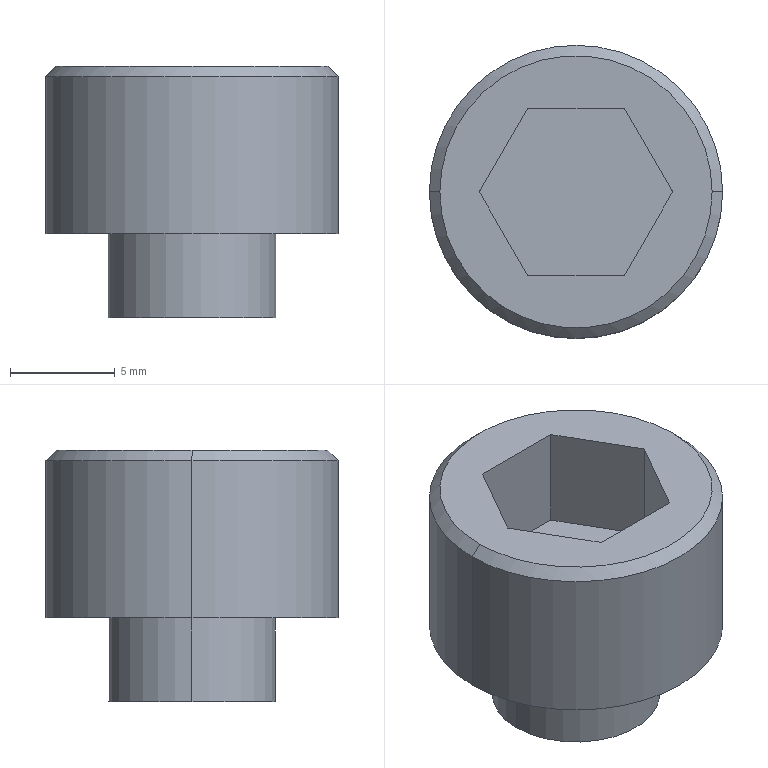Part | NX | 1 solid | 16 faces | box 14 x 14 x 12 mm | volume 1150 mm3 | plane 10 | cylinder 4 | cone 2 | commonest cylinder face diameters 8 x2 14 x2
STEP:
#1=CARTESIAN_POINT('',(6.5,0.,0.));
#2=VERTEX_POINT('',#1);
#3=CARTESIAN_POINT('',(-6.5,0.,0.));
#4=VERTEX_POINT('',#3);
#5=CARTESIAN_POINT('',(0.,0.,0.));
#6=DIRECTION('',(0.,0.,1.));
#7=DIRECTION('',(1.,0.,0.));
#8=AXIS2_PLACEMENT_3D('',#5,#6,#7);
#9=CIRCLE('',#8,6.5);
#10=EDGE_CURVE('',#2,#4,#9,.T.);
#11=ORIENTED_EDGE('',*,*,#10,.F.);
#12=CARTESIAN_POINT('',(7.,0.,-0.5));
#13=VERTEX_POINT('',#12);
#14=CARTESIAN_POINT('',(6.5,0.,0.));
#15=DIRECTION('',(-0.7071,0.,0.7071));
#16=VECTOR('',#15,1.);
#17=LINE('',#14,#16);
#18=EDGE_CURVE('',#13,#2,#17,.T.);
#19=ORIENTED_EDGE('',*,*,#18,.F.);
#20=CARTESIAN_POINT('',(-7.,0.,-0.5));
#21=VERTEX_POINT('',#20);
#22=CARTESIAN_POINT('',(0.,0.,-0.5));
#23=DIRECTION('',(0.,0.,-1.));
#24=DIRECTION('',(1.,0.,0.));
#25=AXIS2_PLACEMENT_3D('',#22,#23,#24);
#26=CIRCLE('',#25,7.);
#27=EDGE_CURVE('',#21,#13,#26,.T.);
#28=ORIENTED_EDGE('',*,*,#27,.F.);
#29=CARTESIAN_POINT('',(-6.5,0.,0.));
#30=DIRECTION('',(0.7071,0.,0.7071));
#31=VECTOR('',#30,1.);
#32=LINE('',#29,#31);
#33=EDGE_CURVE('',#21,#4,#32,.T.);
#34=ORIENTED_EDGE('',*,*,#33,.T.);
#35=EDGE_LOOP('',(#11,#19,#28,#34));
#36=FACE_OUTER_BOUND('',#35,.T.);
#37=CARTESIAN_POINT('',(0.,0.,0.));
#38=DIRECTION('',(0.,0.,-1.));
#39=DIRECTION('',(-1.,0.,0.));
#40=AXIS2_PLACEMENT_3D('',#37,#38,#39);
#41=CONICAL_SURFACE('',#40,6.5,45.);
#42=ADVANCED_FACE('',(#36),#41,.T.);
#43=CARTESIAN_POINT('',(-4.,0.,-12.));
#44=VERTEX_POINT('',#43);
#45=CARTESIAN_POINT('',(4.,0.,-12.));
#46=VERTEX_POINT('',#45);
#47=CARTESIAN_POINT('',(0.,0.,-12.));
#48=DIRECTION('',(0.,0.,-1.));
#49=DIRECTION('',(-1.,0.,0.));
#50=AXIS2_PLACEMENT_3D('',#47,#48,#49);
#51=CIRCLE('',#50,4.);
#52=EDGE_CURVE('',#44,#46,#51,.T.);
#53=ORIENTED_EDGE('',*,*,#52,.F.);
#54=CARTESIAN_POINT('',(-4.,0.,-8.));
#55=VERTEX_POINT('',#54);
#56=CARTESIAN_POINT('',(-4.,0.,-12.));
#57=DIRECTION('',(0.,0.,1.));
#58=VECTOR('',#57,1.);
#59=LINE('',#56,#58);
#60=EDGE_CURVE('',#44,#55,#59,.T.);
#61=ORIENTED_EDGE('',*,*,#60,.T.);
#62=CARTESIAN_POINT('',(4.,0.,-8.));
#63=VERTEX_POINT('',#62);
#64=CARTESIAN_POINT('',(0.,0.,-8.));
#65=DIRECTION('',(0.,0.,-1.));
#66=DIRECTION('',(1.,0.,0.));
#67=AXIS2_PLACEMENT_3D('',#64,#65,#66);
#68=CIRCLE('',#67,4.);
#69=EDGE_CURVE('',#55,#63,#68,.T.);
#70=ORIENTED_EDGE('',*,*,#69,.T.);
#71=CARTESIAN_POINT('',(4.,0.,-12.));
#72=DIRECTION('',(0.,0.,1.));
#73=VECTOR('',#72,1.);
#74=LINE('',#71,#73);
#75=EDGE_CURVE('',#46,#63,#74,.T.);
#76=ORIENTED_EDGE('',*,*,#75,.F.);
#77=EDGE_LOOP('',(#53,#61,#70,#76));
#78=FACE_OUTER_BOUND('',#77,.T.);
#79=CARTESIAN_POINT('',(0.,0.,-12.));
#80=DIRECTION('',(0.,0.,1.));
#81=DIRECTION('',(1.,0.,0.));
#82=AXIS2_PLACEMENT_3D('',#79,#80,#81);
#83=CYLINDRICAL_SURFACE('',#82,4.);
#84=ADVANCED_FACE('',(#78),#83,.T.);
#85=CARTESIAN_POINT('',(7.,0.,-8.));
#86=VERTEX_POINT('',#85);
#87=CARTESIAN_POINT('',(-7.,0.,-8.));
#88=VERTEX_POINT('',#87);
#89=CARTESIAN_POINT('',(0.,0.,-8.));
#90=DIRECTION('',(0.,0.,1.));
#91=DIRECTION('',(1.,0.,0.));
#92=AXIS2_PLACEMENT_3D('',#89,#90,#91);
#93=CIRCLE('',#92,7.);
#94=EDGE_CURVE('',#86,#88,#93,.T.);
#95=ORIENTED_EDGE('',*,*,#94,.T.);
#96=CARTESIAN_POINT('',(-7.,0.,-8.));
#97=DIRECTION('',(0.,0.,1.));
#98=VECTOR('',#97,1.);
#99=LINE('',#96,#98);
#100=EDGE_CURVE('',#88,#21,#99,.T.);
#101=ORIENTED_EDGE('',*,*,#100,.T.);
#102=ORIENTED_EDGE('',*,*,#27,.T.);
#103=CARTESIAN_POINT('',(7.,0.,-8.));
#104=DIRECTION('',(0.,0.,1.));
#105=VECTOR('',#104,1.);
#106=LINE('',#103,#105);
#107=EDGE_CURVE('',#86,#13,#106,.T.);
#108=ORIENTED_EDGE('',*,*,#107,.F.);
#109=EDGE_LOOP('',(#95,#101,#102,#108));
#110=FACE_OUTER_BOUND('',#109,.T.);
#111=CARTESIAN_POINT('',(0.,0.,-8.));
#112=DIRECTION('',(0.,0.,1.));
#113=DIRECTION('',(1.,0.,0.));
#114=AXIS2_PLACEMENT_3D('',#111,#112,#113);
#115=CYLINDRICAL_SURFACE('',#114,7.);
#116=ADVANCED_FACE('',(#110),#115,.T.);
#117=ORIENTED_EDGE('',*,*,#94,.F.);
#118=CARTESIAN_POINT('',(0.,0.,-8.));
#119=DIRECTION('',(0.,0.,1.));
#120=DIRECTION('',(1.,0.,0.));
#121=AXIS2_PLACEMENT_3D('',#118,#119,#120);
#122=CIRCLE('',#121,7.);
#123=EDGE_CURVE('',#88,#86,#122,.T.);
#124=ORIENTED_EDGE('',*,*,#123,.F.);
#125=EDGE_LOOP('',(#117,#124));
#126=FACE_BOUND('',#125,.T.);
#127=CARTESIAN_POINT('',(0.,0.,-8.));
#128=DIRECTION('',(0.,0.,-1.));
#129=DIRECTION('',(1.,0.,0.));
#130=AXIS2_PLACEMENT_3D('',#127,#128,#129);
#131=CIRCLE('',#130,4.);
#132=EDGE_CURVE('',#63,#55,#131,.T.);
#133=ORIENTED_EDGE('',*,*,#132,.F.);
#134=ORIENTED_EDGE('',*,*,#69,.F.);
#135=EDGE_LOOP('',(#133,#134));
#136=FACE_BOUND('',#135,.T.);
#137=CARTESIAN_POINT('',(0.,0.,-8.));
#138=DIRECTION('',(0.,0.,1.));
#139=DIRECTION('',(1.,0.,0.));
#140=AXIS2_PLACEMENT_3D('',#137,#138,#139);
#141=PLANE('',#140);
#142=ADVANCED_FACE('',(#126,#136),#141,.F.);
#143=ORIENTED_EDGE('',*,*,#100,.F.);
#144=ORIENTED_EDGE('',*,*,#123,.T.);
#145=ORIENTED_EDGE('',*,*,#107,.T.);
#146=CARTESIAN_POINT('',(0.,0.,-0.5));
#147=DIRECTION('',(0.,0.,-1.));
#148=DIRECTION('',(1.,0.,0.));
#149=AXIS2_PLACEMENT_3D('',#146,#147,#148);
#150=CIRCLE('',#149,7.);
#151=EDGE_CURVE('',#13,#21,#150,.T.);
#152=ORIENTED_EDGE('',*,*,#151,.T.);
#153=EDGE_LOOP('',(#143,#144,#145,#152));
#154=FACE_OUTER_BOUND('',#153,.T.);
#155=CARTESIAN_POINT('',(0.,0.,-8.));
#156=DIRECTION('',(0.,0.,1.));
#157=DIRECTION('',(1.,0.,0.));
#158=AXIS2_PLACEMENT_3D('',#155,#156,#157);
#159=CYLINDRICAL_SURFACE('',#158,7.);
#160=ADVANCED_FACE('',(#154),#159,.T.);
#161=CARTESIAN_POINT('',(2.309,-4.,0.));
#162=VERTEX_POINT('',#161);
#163=CARTESIAN_POINT('',(4.619,0.,0.));
#164=VERTEX_POINT('',#163);
#165=CARTESIAN_POINT('',(2.309,-4.,0.));
#166=DIRECTION('',(0.5,0.866,0.));
#167=VECTOR('',#166,1.);
#168=LINE('',#165,#167);
#169=EDGE_CURVE('',#162,#164,#168,.T.);
#170=ORIENTED_EDGE('',*,*,#169,.F.);
#171=CARTESIAN_POINT('',(-2.309,-4.,0.));
#172=VERTEX_POINT('',#171);
#173=CARTESIAN_POINT('',(-2.309,-4.,0.));
#174=DIRECTION('',(1.,0.,0.));
#175=VECTOR('',#174,1.);
#176=LINE('',#173,#175);
#177=EDGE_CURVE('',#172,#162,#176,.T.);
#178=ORIENTED_EDGE('',*,*,#177,.F.);
#179=CARTESIAN_POINT('',(-4.619,0.,0.));
#180=VERTEX_POINT('',#179);
#181=CARTESIAN_POINT('',(-4.619,0.,0.));
#182=DIRECTION('',(0.5,-0.866,0.));
#183=VECTOR('',#182,1.);
#184=LINE('',#181,#183);
#185=EDGE_CURVE('',#180,#172,#184,.T.);
#186=ORIENTED_EDGE('',*,*,#185,.F.);
#187=CARTESIAN_POINT('',(-2.309,4.,0.));
#188=VERTEX_POINT('',#187);
#189=CARTESIAN_POINT('',(-2.309,4.,0.));
#190=DIRECTION('',(-0.5,-0.866,0.));
#191=VECTOR('',#190,1.);
#192=LINE('',#189,#191);
#193=EDGE_CURVE('',#188,#180,#192,.T.);
#194=ORIENTED_EDGE('',*,*,#193,.F.);
#195=CARTESIAN_POINT('',(2.309,4.,0.));
#196=VERTEX_POINT('',#195);
#197=CARTESIAN_POINT('',(2.309,4.,0.));
#198=DIRECTION('',(-1.,0.,0.));
#199=VECTOR('',#198,1.);
#200=LINE('',#197,#199);
#201=EDGE_CURVE('',#196,#188,#200,.T.);
#202=ORIENTED_EDGE('',*,*,#201,.F.);
#203=CARTESIAN_POINT('',(4.619,0.,0.));
#204=DIRECTION('',(-0.5,0.866,0.));
#205=VECTOR('',#204,1.);
#206=LINE('',#203,#205);
#207=EDGE_CURVE('',#164,#196,#206,.T.);
#208=ORIENTED_EDGE('',*,*,#207,.F.);
#209=EDGE_LOOP('',(#170,#178,#186,#194,#202,#208));
#210=FACE_BOUND('',#209,.T.);
#211=CARTESIAN_POINT('',(0.,0.,0.));
#212=DIRECTION('',(0.,0.,1.));
#213=DIRECTION('',(1.,0.,0.));
#214=AXIS2_PLACEMENT_3D('',#211,#212,#213);
#215=CIRCLE('',#214,6.5);
#216=EDGE_CURVE('',#4,#2,#215,.T.);
#217=ORIENTED_EDGE('',*,*,#216,.T.);
#218=ORIENTED_EDGE('',*,*,#10,.T.);
#219=EDGE_LOOP('',(#217,#218));
#220=FACE_BOUND('',#219,.T.);
#221=CARTESIAN_POINT('',(0.,0.,0.));
#222=DIRECTION('',(0.,0.,1.));
#223=DIRECTION('',(1.,0.,0.));
#224=AXIS2_PLACEMENT_3D('',#221,#222,#223);
#225=PLANE('',#224);
#226=ADVANCED_FACE('',(#210,#220),#225,.T.);
#227=ORIENTED_EDGE('',*,*,#60,.F.);
#228=CARTESIAN_POINT('',(0.,0.,-12.));
#229=DIRECTION('',(0.,0.,-1.));
#230=DIRECTION('',(-1.,0.,0.));
#231=AXIS2_PLACEMENT_3D('',#228,#229,#230);
#232=CIRCLE('',#231,4.);
#233=EDGE_CURVE('',#46,#44,#232,.T.);
#234=ORIENTED_EDGE('',*,*,#233,.F.);
#235=ORIENTED_EDGE('',*,*,#75,.T.);
#236=ORIENTED_EDGE('',*,*,#132,.T.);
#237=EDGE_LOOP('',(#227,#234,#235,#236));
#238=FACE_OUTER_BOUND('',#237,.T.);
#239=CARTESIAN_POINT('',(0.,0.,-12.));
#240=DIRECTION('',(0.,0.,1.));
#241=DIRECTION('',(1.,0.,0.));
#242=AXIS2_PLACEMENT_3D('',#239,#240,#241);
#243=CYLINDRICAL_SURFACE('',#242,4.);
#244=ADVANCED_FACE('',(#238),#243,.T.);
#245=ORIENTED_EDGE('',*,*,#233,.T.);
#246=ORIENTED_EDGE('',*,*,#52,.T.);
#247=EDGE_LOOP('',(#245,#246));
#248=FACE_OUTER_BOUND('',#247,.T.);
#249=CARTESIAN_POINT('',(0.,0.,-12.));
#250=DIRECTION('',(0.,0.,-1.));
#251=DIRECTION('',(-1.,0.,0.));
#252=AXIS2_PLACEMENT_3D('',#249,#250,#251);
#253=PLANE('',#252);
#254=ADVANCED_FACE('',(#248),#253,.T.);
#255=ORIENTED_EDGE('',*,*,#18,.T.);
#256=ORIENTED_EDGE('',*,*,#216,.F.);
#257=ORIENTED_EDGE('',*,*,#33,.F.);
#258=ORIENTED_EDGE('',*,*,#151,.F.);
#259=EDGE_LOOP('',(#255,#256,#257,#258));
#260=FACE_OUTER_BOUND('',#259,.T.);
#261=CARTESIAN_POINT('',(0.,0.,0.));
#262=DIRECTION('',(0.,0.,-1.));
#263=DIRECTION('',(-1.,0.,0.));
#264=AXIS2_PLACEMENT_3D('',#261,#262,#263);
#265=CONICAL_SURFACE('',#264,6.5,45.);
#266=ADVANCED_FACE('',(#260),#265,.T.);
#267=ORIENTED_EDGE('',*,*,#169,.T.);
#268=CARTESIAN_POINT('',(4.619,0.,-5.));
#269=VERTEX_POINT('',#268);
#270=CARTESIAN_POINT('',(4.619,0.,-5.));
#271=DIRECTION('',(0.,0.,1.));
#272=VECTOR('',#271,1.);
#273=LINE('',#270,#272);
#274=EDGE_CURVE('',#269,#164,#273,.T.);
#275=ORIENTED_EDGE('',*,*,#274,.F.);
#276=CARTESIAN_POINT('',(2.309,-4.,-5.));
#277=VERTEX_POINT('',#276);
#278=CARTESIAN_POINT('',(2.309,-4.,-5.));
#279=DIRECTION('',(0.5,0.866,0.));
#280=VECTOR('',#279,1.);
#281=LINE('',#278,#280);
#282=EDGE_CURVE('',#277,#269,#281,.T.);
#283=ORIENTED_EDGE('',*,*,#282,.F.);
#284=CARTESIAN_POINT('',(2.309,-4.,-5.));
#285=DIRECTION('',(0.,0.,1.));
#286=VECTOR('',#285,1.);
#287=LINE('',#284,#286);
#288=EDGE_CURVE('',#277,#162,#287,.T.);
#289=ORIENTED_EDGE('',*,*,#288,.T.);
#290=EDGE_LOOP('',(#267,#275,#283,#289));
#291=FACE_OUTER_BOUND('',#290,.T.);
#292=CARTESIAN_POINT('',(2.309,-4.,-5.));
#293=DIRECTION('',(0.866,-0.5,0.));
#294=DIRECTION('',(0.5,0.866,0.));
#295=AXIS2_PLACEMENT_3D('',#292,#293,#294);
#296=PLANE('',#295);
#297=ADVANCED_FACE('',(#291),#296,.F.);
#298=ORIENTED_EDGE('',*,*,#177,.T.);
#299=ORIENTED_EDGE('',*,*,#288,.F.);
#300=CARTESIAN_POINT('',(-2.309,-4.,-5.));
#301=VERTEX_POINT('',#300);
#302=CARTESIAN_POINT('',(-2.309,-4.,-5.));
#303=DIRECTION('',(1.,0.,0.));
#304=VECTOR('',#303,1.);
#305=LINE('',#302,#304);
#306=EDGE_CURVE('',#301,#277,#305,.T.);
#307=ORIENTED_EDGE('',*,*,#306,.F.);
#308=CARTESIAN_POINT('',(-2.309,-4.,-5.));
#309=DIRECTION('',(0.,0.,1.));
#310=VECTOR('',#309,1.);
#311=LINE('',#308,#310);
#312=EDGE_CURVE('',#301,#172,#311,.T.);
#313=ORIENTED_EDGE('',*,*,#312,.T.);
#314=EDGE_LOOP('',(#298,#299,#307,#313));
#315=FACE_OUTER_BOUND('',#314,.T.);
#316=CARTESIAN_POINT('',(-2.309,-4.,-5.));
#317=DIRECTION('',(0.,-1.,0.));
#318=DIRECTION('',(0.,0.,-1.));
#319=AXIS2_PLACEMENT_3D('',#316,#317,#318);
#320=PLANE('',#319);
#321=ADVANCED_FACE('',(#315),#320,.F.);
#322=ORIENTED_EDGE('',*,*,#185,.T.);
#323=ORIENTED_EDGE('',*,*,#312,.F.);
#324=CARTESIAN_POINT('',(-4.619,0.,-5.));
#325=VERTEX_POINT('',#324);
#326=CARTESIAN_POINT('',(-4.619,0.,-5.));
#327=DIRECTION('',(0.5,-0.866,0.));
#328=VECTOR('',#327,1.);
#329=LINE('',#326,#328);
#330=EDGE_CURVE('',#325,#301,#329,.T.);
#331=ORIENTED_EDGE('',*,*,#330,.F.);
#332=CARTESIAN_POINT('',(-4.619,0.,-5.));
#333=DIRECTION('',(0.,0.,1.));
#334=VECTOR('',#333,1.);
#335=LINE('',#332,#334);
#336=EDGE_CURVE('',#325,#180,#335,.T.);
#337=ORIENTED_EDGE('',*,*,#336,.T.);
#338=EDGE_LOOP('',(#322,#323,#331,#337));
#339=FACE_OUTER_BOUND('',#338,.T.);
#340=CARTESIAN_POINT('',(-4.619,0.,-5.));
#341=DIRECTION('',(-0.866,-0.5,0.));
#342=DIRECTION('',(0.5,-0.866,0.));
#343=AXIS2_PLACEMENT_3D('',#340,#341,#342);
#344=PLANE('',#343);
#345=ADVANCED_FACE('',(#339),#344,.F.);
#346=ORIENTED_EDGE('',*,*,#193,.T.);
#347=ORIENTED_EDGE('',*,*,#336,.F.);
#348=CARTESIAN_POINT('',(-2.309,4.,-5.));
#349=VERTEX_POINT('',#348);
#350=CARTESIAN_POINT('',(-2.309,4.,-5.));
#351=DIRECTION('',(-0.5,-0.866,0.));
#352=VECTOR('',#351,1.);
#353=LINE('',#350,#352);
#354=EDGE_CURVE('',#349,#325,#353,.T.);
#355=ORIENTED_EDGE('',*,*,#354,.F.);
#356=CARTESIAN_POINT('',(-2.309,4.,-5.));
#357=DIRECTION('',(0.,0.,1.));
#358=VECTOR('',#357,1.);
#359=LINE('',#356,#358);
#360=EDGE_CURVE('',#349,#188,#359,.T.);
#361=ORIENTED_EDGE('',*,*,#360,.T.);
#362=EDGE_LOOP('',(#346,#347,#355,#361));
#363=FACE_OUTER_BOUND('',#362,.T.);
#364=CARTESIAN_POINT('',(-2.309,4.,-5.));
#365=DIRECTION('',(-0.866,0.5,0.));
#366=DIRECTION('',(-0.5,-0.866,0.));
#367=AXIS2_PLACEMENT_3D('',#364,#365,#366);
#368=PLANE('',#367);
#369=ADVANCED_FACE('',(#363),#368,.F.);
#370=ORIENTED_EDGE('',*,*,#201,.T.);
#371=ORIENTED_EDGE('',*,*,#360,.F.);
#372=CARTESIAN_POINT('',(2.309,4.,-5.));
#373=VERTEX_POINT('',#372);
#374=CARTESIAN_POINT('',(2.309,4.,-5.));
#375=DIRECTION('',(-1.,0.,0.));
#376=VECTOR('',#375,1.);
#377=LINE('',#374,#376);
#378=EDGE_CURVE('',#373,#349,#377,.T.);
#379=ORIENTED_EDGE('',*,*,#378,.F.);
#380=CARTESIAN_POINT('',(2.309,4.,-5.));
#381=DIRECTION('',(0.,0.,1.));
#382=VECTOR('',#381,1.);
#383=LINE('',#380,#382);
#384=EDGE_CURVE('',#373,#196,#383,.T.);
#385=ORIENTED_EDGE('',*,*,#384,.T.);
#386=EDGE_LOOP('',(#370,#371,#379,#385));
#387=FACE_OUTER_BOUND('',#386,.T.);
#388=CARTESIAN_POINT('',(2.309,4.,-5.));
#389=DIRECTION('',(0.,1.,0.));
#390=DIRECTION('',(-1.,0.,0.));
#391=AXIS2_PLACEMENT_3D('',#388,#389,#390);
#392=PLANE('',#391);
#393=ADVANCED_FACE('',(#387),#392,.F.);
#394=ORIENTED_EDGE('',*,*,#207,.T.);
#395=ORIENTED_EDGE('',*,*,#384,.F.);
#396=CARTESIAN_POINT('',(4.619,0.,-5.));
#397=DIRECTION('',(-0.5,0.866,0.));
#398=VECTOR('',#397,1.);
#399=LINE('',#396,#398);
#400=EDGE_CURVE('',#269,#373,#399,.T.);
#401=ORIENTED_EDGE('',*,*,#400,.F.);
#402=ORIENTED_EDGE('',*,*,#274,.T.);
#403=EDGE_LOOP('',(#394,#395,#401,#402));
#404=FACE_OUTER_BOUND('',#403,.T.);
#405=CARTESIAN_POINT('',(4.619,0.,-5.));
#406=DIRECTION('',(0.866,0.5,0.));
#407=DIRECTION('',(-0.5,0.866,0.));
#408=AXIS2_PLACEMENT_3D('',#405,#406,#407);
#409=PLANE('',#408);
#410=ADVANCED_FACE('',(#404),#409,.F.);
#411=ORIENTED_EDGE('',*,*,#282,.T.);
#412=ORIENTED_EDGE('',*,*,#400,.T.);
#413=ORIENTED_EDGE('',*,*,#378,.T.);
#414=ORIENTED_EDGE('',*,*,#354,.T.);
#415=ORIENTED_EDGE('',*,*,#330,.T.);
#416=ORIENTED_EDGE('',*,*,#306,.T.);
#417=EDGE_LOOP('',(#411,#412,#413,#414,#415,#416));
#418=FACE_OUTER_BOUND('',#417,.T.);
#419=CARTESIAN_POINT('',(0.,0.,-5.));
#420=DIRECTION('',(0.,0.,1.));
#421=DIRECTION('',(1.,0.,0.));
#422=AXIS2_PLACEMENT_3D('',#419,#420,#421);
#423=PLANE('',#422);
#424=ADVANCED_FACE('',(#418),#423,.T.);
#425=CLOSED_SHELL('',(#42,#84,#116,#142,#160,#226,#244,#254,#266,#297,#321,#345,#369,#393,#410,#424));
#426=MANIFOLD_SOLID_BREP('',#425);
#427=(LENGTH_UNIT()NAMED_UNIT(*)SI_UNIT(.MILLI.,.METRE.));
#428=UNCERTAINTY_MEASURE_WITH_UNIT(LENGTH_MEASURE(0.00002),#427,'','');
#429=(NAMED_UNIT(*)PLANE_ANGLE_UNIT()SI_UNIT($,.RADIAN.));
#430=PLANE_ANGLE_MEASURE_WITH_UNIT(PLANE_ANGLE_MEASURE(0.01745),#429);
#431=DIMENSIONAL_EXPONENTS(0.,0.,0.,0.,0.,0.,0.);
#432=(CONVERSION_BASED_UNIT('DEGREE',#430)NAMED_UNIT(#431)PLANE_ANGLE_UNIT());
#433=(NAMED_UNIT(*)SI_UNIT($,.STERADIAN.)SOLID_ANGLE_UNIT());
#434=(GEOMETRIC_REPRESENTATION_CONTEXT(3)GLOBAL_UNCERTAINTY_ASSIGNED_CONTEXT((#428))GLOBAL_UNIT_ASSIGNED_CONTEXT((#427,#432,#433))REPRESENTATION_CONTEXT('',''));
#435=ADVANCED_BREP_SHAPE_REPRESENTATION('',(#426),#434);